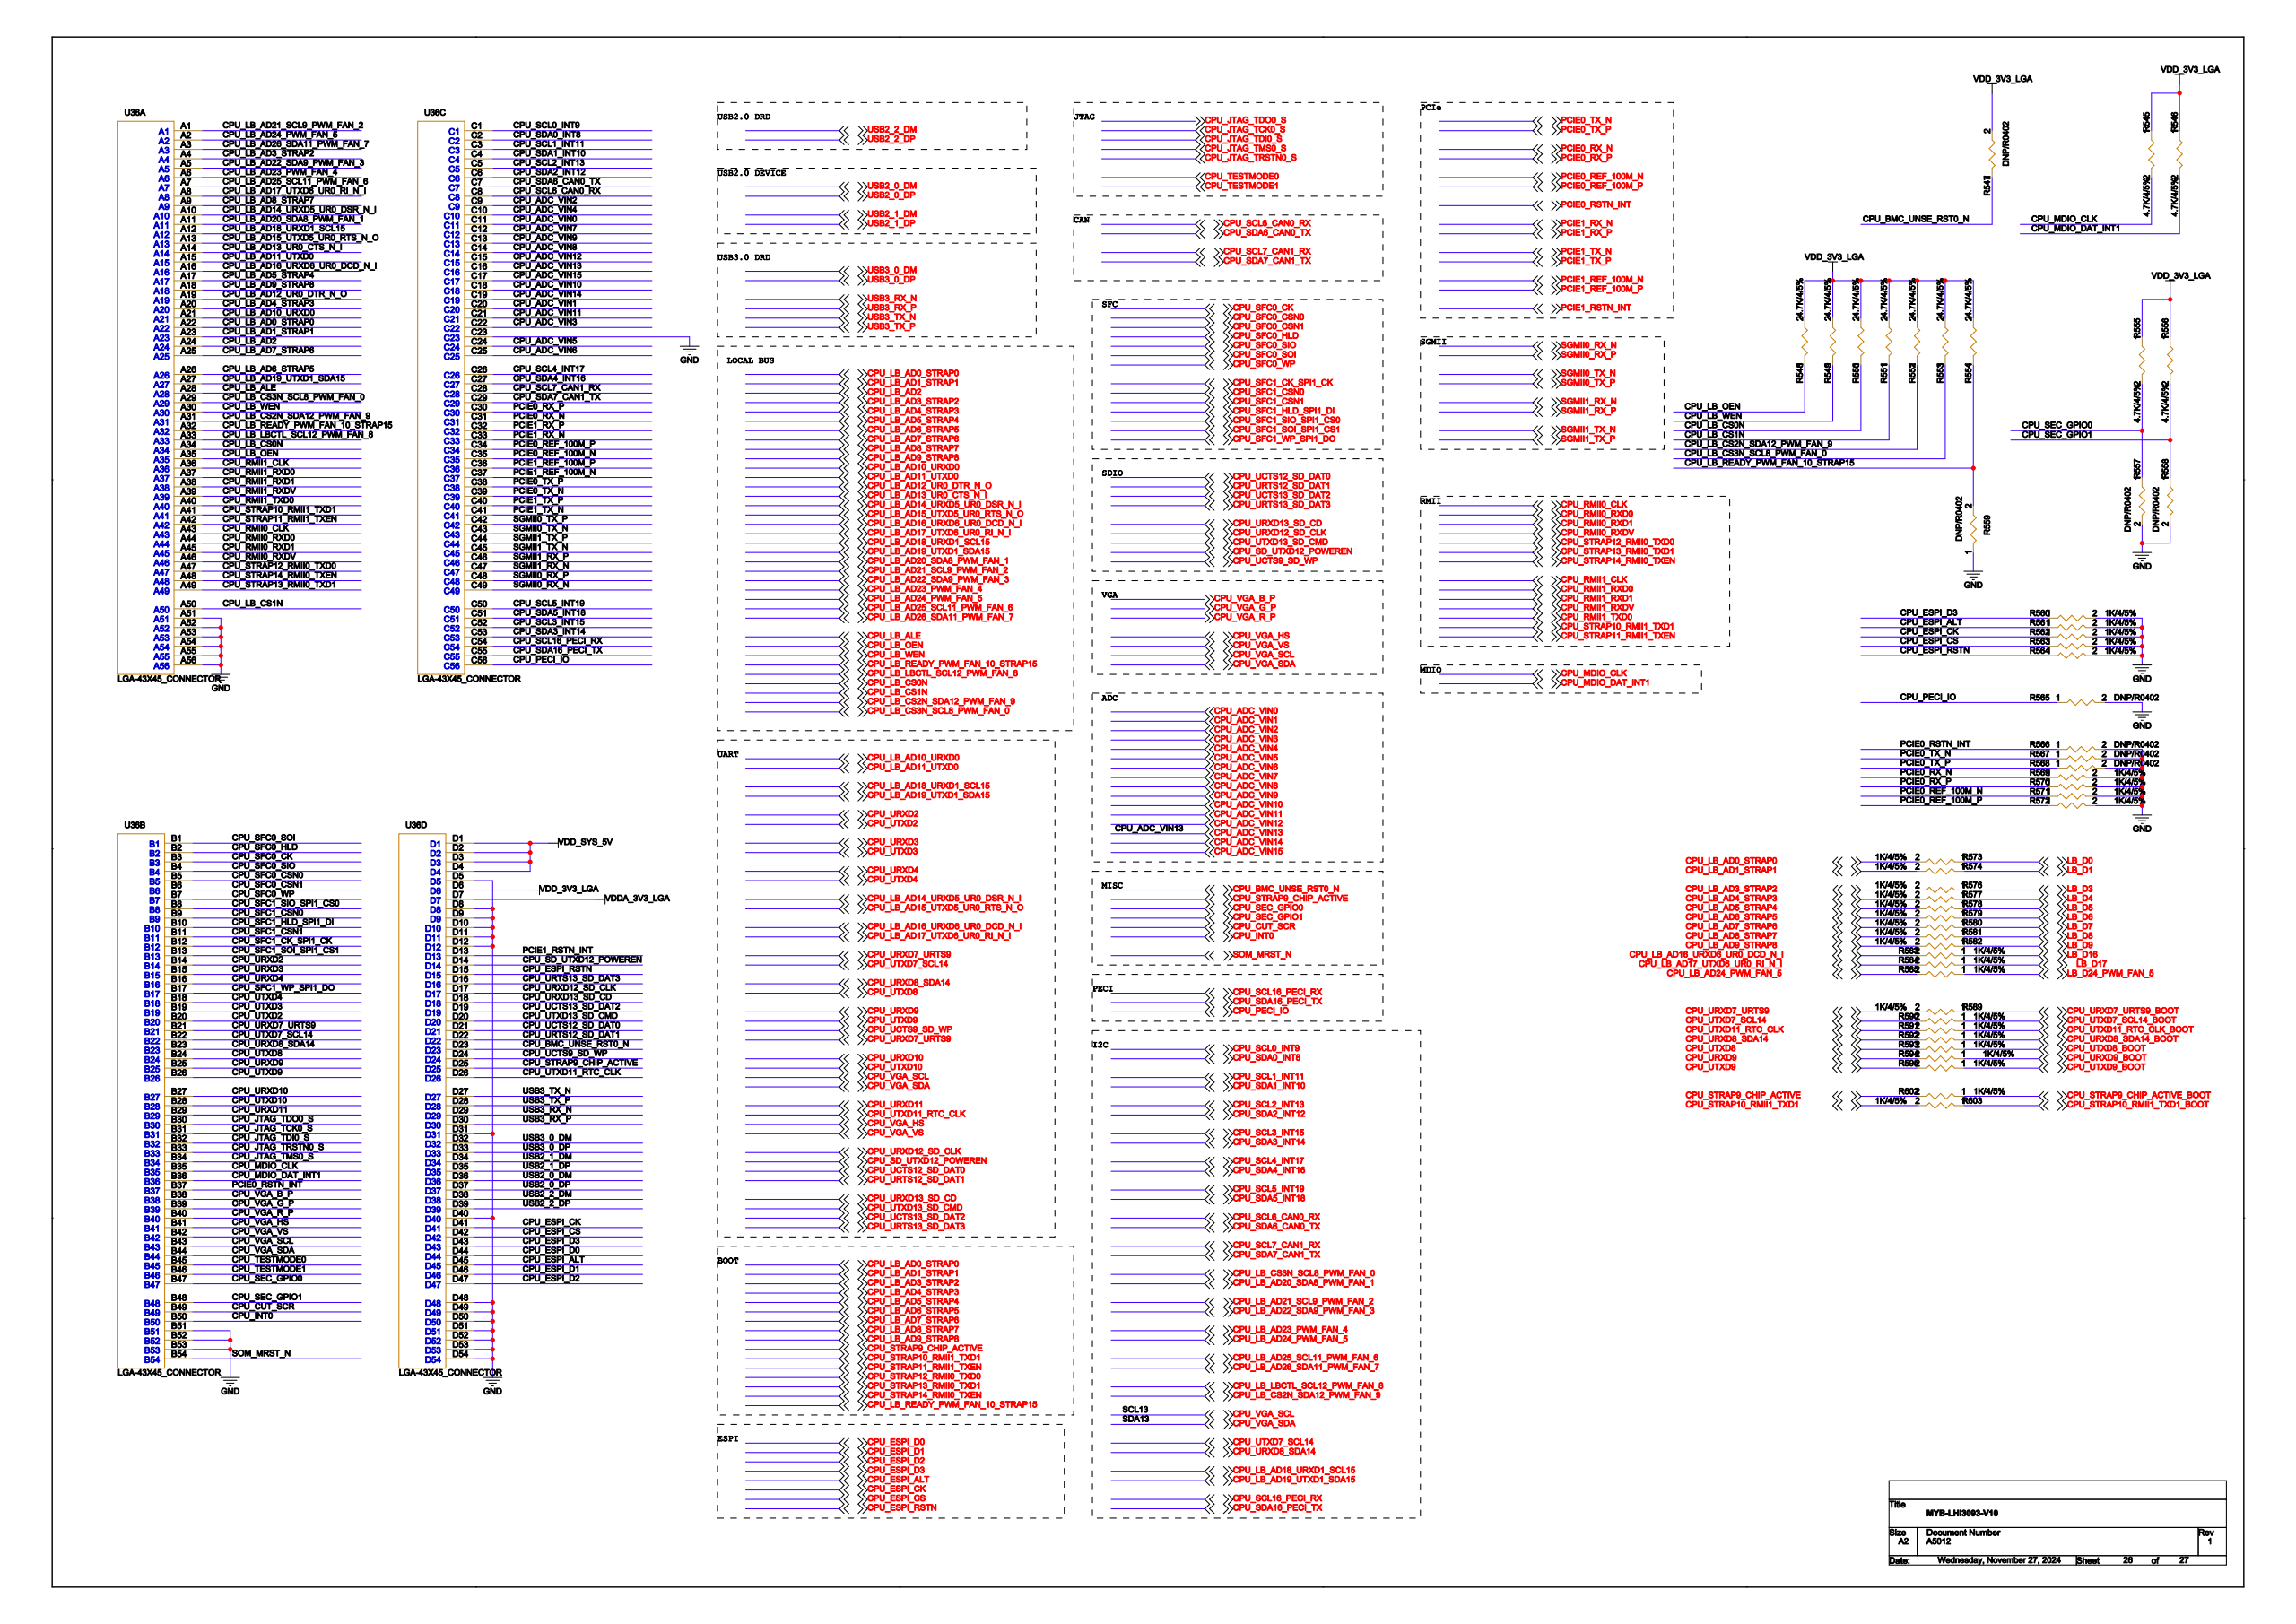Circuit board | Cadence Allegro | 1159 parts | 708 nets | one sheet of the schematic
Parts on this sheet (reference | value | footprint):
D46 | B72590D50H160 | D0402
D47 | B72590D50H160 | D0402
D48 | B72590D50H160 | D0402
D49 | B72590D50H160 | D0402
D50 | DNP | D0402
D51 | B72590D50H160 | D0402
D52 | B72590D50H160 | D0402
D53 | B72590D50H160 | D0402
D54 | B72590D50H160 | D0402
R545 | 4.7K/4/5% | R0402
R546 | 4.7K/4/5% | R0402
R547 | DNP/R0402 | R0402
R548 | 4.7K/4/5% | R0402
R549 | 4.7K/4/5% | R0402
R550 | 4.7K/4/5% | R0402
R551 | 4.7K/4/5% | R0402
R552 | 4.7K/4/5% | R0402
R553 | 4.7K/4/5% | R0402
R554 | 4.7K/4/5% | R0402
R555 | 4.7K/4/5% | R0402
R556 | 4.7K/4/5% | R0402
R557 | DNP/R0402 | R0402
R558 | DNP/R0402 | R0402
R559 | DNP/R0402 | R0402
R565 | DNP/R0402 | R0402
R566 | DNP/R0402 | R0402
R567 | DNP/R0402 | R0402
R568 | DNP/R0402 | R0402
U36 | LGA-43X45_CONNECTOR | SMD-LGA-43X45-3
Nets of these parts (net: part-pin ...):
GND: D46-1 D47-1 D48-1 D49-1 D50-1 D51-1 D52-1 D53-1 D54-1 R557-2 R558-2 R559-1 R565-2 R566-2 R567-2 R568-2 U36-A51 U36-A52 U36-A53 U36-A54 U36-A55 U36-A56 U36-B51 U36-B52 U36-B53 U36-C23 U36-D5 U36-D8 U36-D9 U36-D10 U36-D11 U36-D12 U36-D31 U36-D40 U36-D48 U36-D49 U36-D50 U36-D51 U36-D52 U36-D53 U36-D54
VDD_SYS_5V: U36-D1 U36-D2 U36-D3 U36-D4
CPU_ESPI_D0: U36-D44
CPU_ESPI_D1: U36-D46
N14961789: D46-2
PCIE1_RSTN_INT: U36-D13
PCIE1_REF_100M_P: U36-C36
PCIE1_REF_100M_N: U36-C37
PCIE0_REF_100M_P: U36-C34
PCIE0_REF_100M_N: U36-C35
SOM_MRST_N: U36-B54
CPU_JTAG_TMS0_S: U36-B34
ANT: D50-2
N14960565: D47-2
N14960569: D48-2
N14960573: D49-2
SGMII0_TX_N: U36-C43
SGMII0_TX_P: U36-C42
SGMII1_TX_N: U36-C45
SGMII1_TX_P: U36-C44
CPU_ADC_VIN0: U36-C11
CPU_ADC_VIN8: U36-C14
CPU_ADC_VIN1: U36-C20
CPU_ADC_VIN9: U36-C13
CPU_ADC_VIN2: U36-C9
CPU_ADC_VIN10: U36-C18
CPU_ADC_VIN3: U36-C22
CPU_ADC_VIN11: U36-C21
CPU_ADC_VIN4: U36-C10
CPU_ADC_VIN12: U36-C15
CPU_ADC_VIN5: U36-C24
CPU_ADC_VIN13: U36-C16
CPU_ADC_VIN6: U36-C25
CPU_ADC_VIN14: U36-C19
CPU_ADC_VIN7: U36-C12
CPU_ADC_VIN15: U36-C17
CPU_SFC1_HLD_SPI1_DI: U36-B10
CPU_SFC1_SIO_SPI1_CS0: U36-B8
CPU_SFC1_CSN0: U36-B9
USB2_0_DP: U36-D37
USB2_0_DM: U36-D36
USB2_1_DP: U36-D35
USB2_1_DM: U36-D34
N14964581: D51-2
RGMII1_LED_ACT: D52-2
RGMII1_LED_LINK: D53-2
RGMII2_LED_ACT: D54-2
VDD_3V3_LGA: R545-1 R546-1 R547-2 R548-2 R549-2 R550-2 R551-2 R552-2 R553-2 R554-2 R555-1 R556-1 U36-D6
CPU_SFC0_CSN1: U36-B6
CPU_LB_AD22_SDA9_PWM_FAN_3: U36-A5
CPU_LB_AD23_PWM_FAN_4: U36-A6
CPU_LB_AD25_SCL11_PWM_FAN_6: U36-A7
CPU_LB_AD26_SDA11_PWM_FAN_7: U36-A3
CPU_LB_AD18_URXD1_SCL15: U36-A12
CPU_LB_ALE: U36-A28
CPU_LB_AD10_URXD0: U36-A21
CPU_LB_OEN: R548-1 U36-A35
CPU_LB_AD11_UTXD0: U36-A15
CPU_LB_WEN: R549-1 U36-A30
CPU_LB_AD12_UR0_DTR_N_O: U36-A19
CPU_LB_READY_PWM_FAN_10_STRAP15: R554-1 R559-2 U36-A32
CPU_LB_AD13_UR0_CTS_N_I: U36-A14
CPU_LB_LBCTL_SCL12_PWM_FAN_8: U36-A33
CPU_LB_AD14_URXD5_UR0_DSR_N_I: U36-A10
CPU_LB_CS0N: R550-1 U36-A34
CPU_LB_AD15_UTXD5_UR0_RTS_N_O: U36-A13
CPU_LB_CS1N: R551-1 U36-A50
CPU_LB_CS2N_SDA12_PWM_FAN_9: R552-1 U36-A31
CPU_LB_CS3N_SCL8_PWM_FAN_0: R553-1 U36-A29
CPU_LB_AD19_UTXD1_SDA15: U36-A27
CPU_LB_AD2: U36-A24
CPU_LB_AD20_SDA8_PWM_FAN_1: U36-A11
CPU_LB_AD21_SCL9_PWM_FAN_2: U36-A1
CPU_SCL5_INT19: U36-C50
CPU_URXD8_SDA14: U36-B23
CPU_UTXD8: U36-B24
CPU_SCL2_INT13: U36-C5
CPU_URXD9: U36-B25
CPU_SDA2_INT12: U36-C6
CPU_UTXD9: U36-B26
CPU_SCL0_INT9: U36-C1
CPU_SCL3_INT15: U36-C52
CPU_SDA3_INT14: U36-C53
CPU_SCL4_INT17: U36-C26
CPU_SDA4_INT16: U36-C27
CPU_SDA5_INT18: U36-C51
CPU_SDA0_INT8: U36-C2
CPU_SCL1_INT11: U36-C3
CPU_SDA1_INT10: U36-C4
CPU_SFC0_CSN0: U36-B5
CPU_SFC0_CK: U36-B3
CPU_SFC0_SIO: U36-B4
CPU_SFC0_SOI: U36-B1
CPU_SFC0_WP: U36-B7
CPU_JTAG_TDO0_S: U36-B30
CPU_JTAG_TRSTN0_S: U36-B33
CPU_JTAG_TDI0_S: U36-B32
PCIE1_TX_N: U36-C41
PCIE1_TX_P: U36-C40
USB3_RX_P: U36-D30
USB3_RX_N: U36-D29
USB3_TX_P: U36-D28
USB3_TX_N: U36-D27
USB3_0_DM: U36-D32
USB3_0_DP: U36-D33
CPU_SD_UTXD12_POWEREN: U36-D14
CPU_JTAG_TCK0_S: U36-B31
CPU_SFC0_HLD: U36-B2
USB2_2_DM: U36-D38
USB2_2_DP: U36-D39
PCIE1_RX_P: U36-C32
PCIE1_RX_N: U36-C33
CPU_URXD2: U36-B14
CPU_URXD4: U36-B16
CPU_UTXD2: U36-B20
CPU_UTXD4: U36-B18
CPU_SDA6_CAN0_TX: U36-C7
CPU_SCL6_CAN0_RX: U36-C8
CPU_SDA7_CAN1_TX: U36-C29
CPU_SCL7_CAN1_RX: U36-C28
CPU_INT0: U36-B50
CPU_SFC1_SOI_SPI1_CS1: U36-B13
CPU_SFC1_WP_SPI1_DO: U36-B17
CPU_SFC1_CSN1: U36-B11
CPU_STRAP9_CHIP_ACTIVE: U36-D25
CPU_LB_AD24_PWM_FAN_5: U36-A2
CPU_ESPI_D3: U36-D43
CPU_ESPI_ALT: U36-D45
CPU_ESPI_CK: U36-D41
CPU_ESPI_CS: U36-D42
CPU_ESPI_RSTN: U36-D15
PCIE0_RX_N: U36-C31
PCIE0_RX_P: U36-C30
CPU_LB_AD0_STRAP0: U36-A22
CPU_LB_AD1_STRAP1: U36-A23
CPU_LB_AD3_STRAP2: U36-A4
CPU_LB_AD4_STRAP3: U36-A20
CPU_LB_AD5_STRAP4: U36-A17
CPU_LB_AD6_STRAP5: U36-A26
CPU_LB_AD7_STRAP6: U36-A25
CPU_LB_AD8_STRAP7: U36-A9
CPU_LB_AD9_STRAP8: U36-A18
CPU_LB_AD16_URXD6_UR0_DCD_N_I: U36-A16
CPU_LB_AD17_UTXD6_UR0_RI_N_I: U36-A8
CPU_URXD7_URTS9: U36-B21
CPU_UTXD7_SCL14: U36-B22
CPU_UTXD11_RTC_CLK: U36-D26
CPU_STRAP10_RMII1_TXD1: U36-A41
CPU_SDA16_PECI_TX: U36-C55
CPU_UCTS9_SD_WP: U36-D24
CPU_SCL16_PECI_RX: U36-C54
CPU_UCTS13_SD_DAT2: U36-D19
CPU_URTS13_SD_DAT3: U36-D16
CPU_UTXD13_SD_CMD: U36-D20
CPU_URXD12_SD_CLK: U36-D17
CPU_UCTS12_SD_DAT0: U36-D21
CPU_URTS12_SD_DAT1: U36-D22
CPU_URXD13_SD_CD: U36-D18
CPU_MDIO_CLK: R545-2 U36-B35
CPU_MDIO_DAT_INT1: R546-2 U36-B36
CPU_BMC_UNSE_RST0_N: R547-1 U36-D23
CPU_RMII0_CLK: U36-A43
CPU_STRAP14_RMII0_TXEN: U36-A48
CPU_STRAP12_RMII0_TXD0: U36-A47
CPU_STRAP13_RMII0_TXD1: U36-A49
CPU_RMII0_RXD0: U36-A44
CPU_RMII0_RXD1: U36-A45
CPU_RMII1_CLK: U36-A36
CPU_STRAP11_RMII1_TXEN: U36-A42
CPU_RMII1_TXD0: U36-A40
CPU_RMII1_RXD0: U36-A37
CPU_RMII1_RXD1: U36-A38
CPU_UTXD3: U36-B19
CPU_URXD3: U36-B15
CPU_URXD11: U36-B29
CPU_CUT_SCR: U36-B49
CPU_URXD10: U36-B27
CPU_UTXD10: U36-B28
CPU_SFC1_CK_SPI1_CK: U36-B12
CPU_TESTMODE1: U36-B46
CPU_TESTMODE0: U36-B45
CPU_SEC_GPIO0: R555-2 R557-1 U36-B47
CPU_SEC_GPIO1: R556-2 R558-1 U36-B48
CPU_VGA_SDA: U36-B44
CPU_VGA_SCL: U36-B43
CPU_PECI_IO: R565-1 U36-C56
PCIE0_RSTN_INT: R566-1 U36-B37
PCIE0_TX_N: R567-1 U36-C39
PCIE0_TX_P: R568-1 U36-C38
CPU_RMII0_RXDV: U36-A46
CPU_RMII1_RXDV: U36-A39
VDDA_3V3_LGA: U36-D7
CPU_VGA_B_P: U36-B38
CPU_VGA_G_P: U36-B39
CPU_VGA_R_P: U36-B40
CPU_VGA_VS: U36-B42
CPU_VGA_HS: U36-B41
CPU_ESPI_D2: U36-D47
SGMII0_RX_N: U36-C49
SGMII0_RX_P: U36-C48
SGMII1_RX_N: U36-C47
SGMII1_RX_P: U36-C46